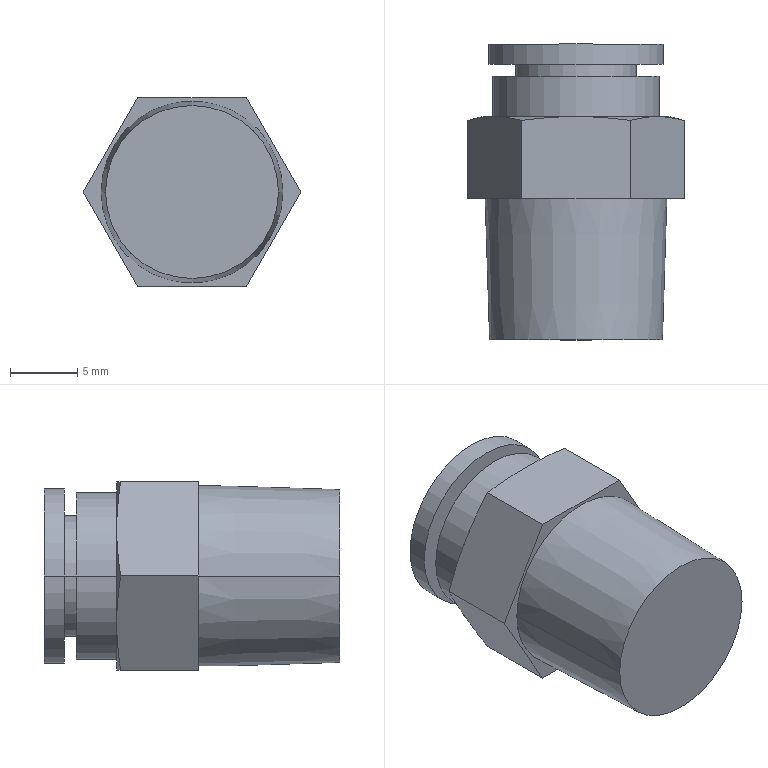Part | STEP file | upright fitting KQ2H08-02AS | 1 solid | 30 faces | box 16.166 x 22 x 14 mm | volume 2374 mm3 | plane 13 | cone 9 | cylinder 8 | commonest cylinder face diameters 8 x2 8.95 x2 12.4 x2 13 x2